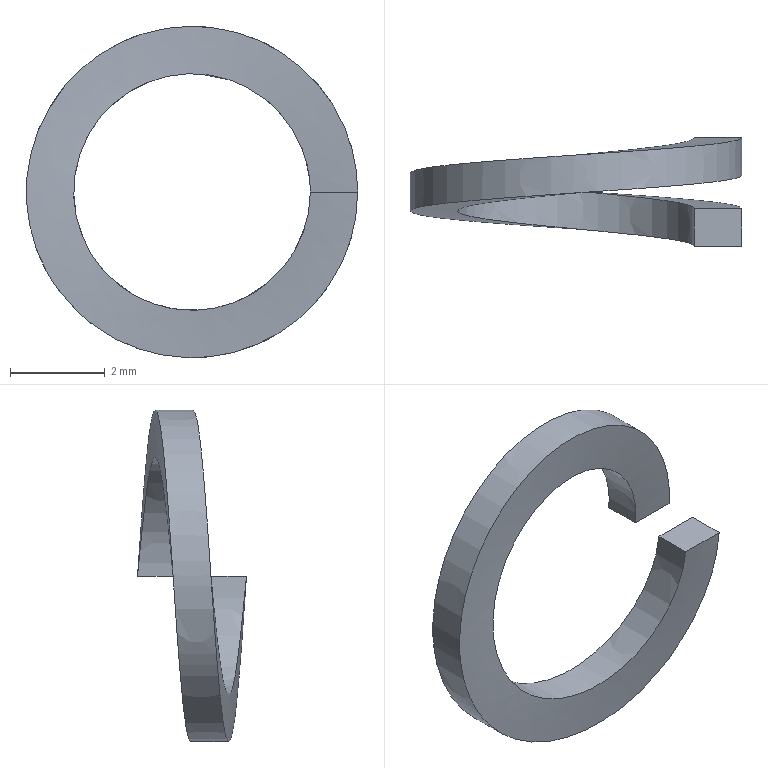Part | STEP file | _X2_751F4E45_X0_MS731-1_X2_8_17 | 1 solid | 6 faces | box 7 x 2.3 x 7 mm | volume 15.077 mm3 | spline 4 | plane 2